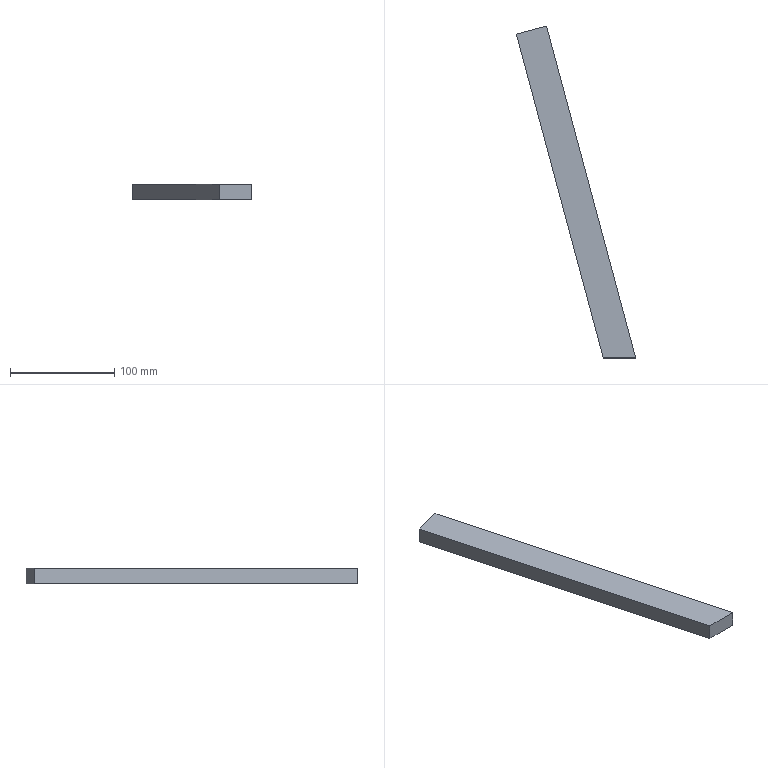Part | NX | features solid 2 | 1 solid | 6 faces | box 114.337 x 318.565 x 15 mm | volume 146602 mm3 | plane 6
STEP:
#1=CARTESIAN_POINT('',(-430.083,270.,-115.));
#2=VERTEX_POINT('',#1);
#3=CARTESIAN_POINT('',(-513.362,580.8,-115.));
#4=VERTEX_POINT('',#3);
#5=CARTESIAN_POINT('',(-443.481,320.,-115.));
#6=DIRECTION('',(-0.2588,0.9659,0.));
#7=VECTOR('',#6,1000.);
#8=LINE('',#5,#7);
#9=EDGE_CURVE('',#2,#4,#8,.T.);
#10=ORIENTED_EDGE('',*,*,#9,.F.);
#11=CARTESIAN_POINT('',(-430.083,270.,-100.));
#12=VERTEX_POINT('',#11);
#13=CARTESIAN_POINT('',(-430.083,270.,-100.));
#14=DIRECTION('',(0.,0.,1.));
#15=VECTOR('',#14,1000.);
#16=LINE('',#13,#15);
#17=EDGE_CURVE('',#2,#12,#16,.T.);
#18=ORIENTED_EDGE('',*,*,#17,.T.);
#19=CARTESIAN_POINT('',(-513.362,580.8,-100.));
#20=VERTEX_POINT('',#19);
#21=CARTESIAN_POINT('',(-443.481,320.,-100.));
#22=DIRECTION('',(-0.2588,0.9659,0.));
#23=VECTOR('',#22,1000.);
#24=LINE('',#21,#23);
#25=EDGE_CURVE('',#12,#20,#24,.T.);
#26=ORIENTED_EDGE('',*,*,#25,.T.);
#27=CARTESIAN_POINT('',(-513.362,580.8,-100.));
#28=DIRECTION('',(0.,0.,-1.));
#29=VECTOR('',#28,1000.);
#30=LINE('',#27,#29);
#31=EDGE_CURVE('',#4,#20,#30,.F.);
#32=ORIENTED_EDGE('',*,*,#31,.F.);
#33=EDGE_LOOP('',(#10,#18,#26,#32));
#34=FACE_BOUND('',#33,.T.);
#35=CARTESIAN_POINT('',(-443.481,320.,-115.));
#36=DIRECTION('',(-0.9659,-0.2588,0.));
#37=DIRECTION('',(0.,0.,1.));
#38=AXIS2_PLACEMENT_3D('',#35,#36,#37);
#39=PLANE('',#38);
#40=ADVANCED_FACE('',(#34),#39,.T.);
#41=ORIENTED_EDGE('',*,*,#25,.F.);
#42=CARTESIAN_POINT('',(-399.025,270.,-100.));
#43=VERTEX_POINT('',#42);
#44=CARTESIAN_POINT('',(-442.5,270.,-100.));
#45=DIRECTION('',(1.,0.,0.));
#46=VECTOR('',#45,1000.);
#47=LINE('',#44,#46);
#48=EDGE_CURVE('',#12,#43,#47,.T.);
#49=ORIENTED_EDGE('',*,*,#48,.T.);
#50=CARTESIAN_POINT('',(-484.384,588.565,-100.));
#51=VERTEX_POINT('',#50);
#52=CARTESIAN_POINT('',(-414.503,327.765,-100.));
#53=DIRECTION('',(-0.2588,0.9659,0.));
#54=VECTOR('',#53,1000.);
#55=LINE('',#52,#54);
#56=EDGE_CURVE('',#43,#51,#55,.T.);
#57=ORIENTED_EDGE('',*,*,#56,.T.);
#58=CARTESIAN_POINT('',(-513.362,580.8,-100.));
#59=DIRECTION('',(-0.9659,-0.2588,0.));
#60=VECTOR('',#59,1000.);
#61=LINE('',#58,#60);
#62=EDGE_CURVE('',#20,#51,#61,.F.);
#63=ORIENTED_EDGE('',*,*,#62,.F.);
#64=EDGE_LOOP('',(#41,#49,#57,#63));
#65=FACE_BOUND('',#64,.T.);
#66=CARTESIAN_POINT('',(-443.481,320.,-100.));
#67=DIRECTION('',(0.,0.,1.));
#68=DIRECTION('',(0.9659,0.2588,0.));
#69=AXIS2_PLACEMENT_3D('',#66,#67,#68);
#70=PLANE('',#69);
#71=ADVANCED_FACE('',(#65),#70,.T.);
#72=ORIENTED_EDGE('',*,*,#56,.F.);
#73=CARTESIAN_POINT('',(-399.025,270.,-115.));
#74=VERTEX_POINT('',#73);
#75=CARTESIAN_POINT('',(-399.025,270.,-115.));
#76=DIRECTION('',(0.,0.,-1.));
#77=VECTOR('',#76,1000.);
#78=LINE('',#75,#77);
#79=EDGE_CURVE('',#74,#43,#78,.F.);
#80=ORIENTED_EDGE('',*,*,#79,.F.);
#81=CARTESIAN_POINT('',(-484.384,588.565,-115.));
#82=VERTEX_POINT('',#81);
#83=CARTESIAN_POINT('',(-414.503,327.765,-115.));
#84=DIRECTION('',(-0.2588,0.9659,0.));
#85=VECTOR('',#84,1000.);
#86=LINE('',#83,#85);
#87=EDGE_CURVE('',#74,#82,#86,.T.);
#88=ORIENTED_EDGE('',*,*,#87,.T.);
#89=CARTESIAN_POINT('',(-484.384,588.565,-115.));
#90=DIRECTION('',(0.,0.,1.));
#91=VECTOR('',#90,1000.);
#92=LINE('',#89,#91);
#93=EDGE_CURVE('',#82,#51,#92,.T.);
#94=ORIENTED_EDGE('',*,*,#93,.T.);
#95=EDGE_LOOP('',(#72,#80,#88,#94));
#96=FACE_BOUND('',#95,.T.);
#97=CARTESIAN_POINT('',(-414.503,327.765,-115.));
#98=DIRECTION('',(-0.9659,-0.2588,0.));
#99=DIRECTION('',(0.,0.,1.));
#100=AXIS2_PLACEMENT_3D('',#97,#98,#99);
#101=PLANE('',#100);
#102=ADVANCED_FACE('',(#96),#101,.F.);
#103=CARTESIAN_POINT('',(-443.481,270.,-115.));
#104=DIRECTION('',(-1.,0.,0.));
#105=VECTOR('',#104,1000.);
#106=LINE('',#103,#105);
#107=EDGE_CURVE('',#2,#74,#106,.F.);
#108=ORIENTED_EDGE('',*,*,#107,.F.);
#109=ORIENTED_EDGE('',*,*,#9,.T.);
#110=CARTESIAN_POINT('',(-513.362,580.8,-115.));
#111=DIRECTION('',(0.9659,0.2588,0.));
#112=VECTOR('',#111,1000.);
#113=LINE('',#110,#112);
#114=EDGE_CURVE('',#4,#82,#113,.T.);
#115=ORIENTED_EDGE('',*,*,#114,.T.);
#116=ORIENTED_EDGE('',*,*,#87,.F.);
#117=EDGE_LOOP('',(#108,#109,#115,#116));
#118=FACE_BOUND('',#117,.T.);
#119=CARTESIAN_POINT('',(-443.481,320.,-115.));
#120=DIRECTION('',(0.,0.,1.));
#121=DIRECTION('',(0.9659,0.2588,0.));
#122=AXIS2_PLACEMENT_3D('',#119,#120,#121);
#123=PLANE('',#122);
#124=ADVANCED_FACE('',(#118),#123,.F.);
#125=ORIENTED_EDGE('',*,*,#93,.F.);
#126=ORIENTED_EDGE('',*,*,#114,.F.);
#127=ORIENTED_EDGE('',*,*,#31,.T.);
#128=ORIENTED_EDGE('',*,*,#62,.T.);
#129=EDGE_LOOP('',(#125,#126,#127,#128));
#130=FACE_BOUND('',#129,.T.);
#131=CARTESIAN_POINT('',(-513.362,580.8,-100.));
#132=DIRECTION('',(0.2588,-0.9659,0.));
#133=DIRECTION('',(0.9659,0.2588,0.));
#134=AXIS2_PLACEMENT_3D('',#131,#132,#133);
#135=PLANE('',#134);
#136=ADVANCED_FACE('',(#130),#135,.F.);
#137=ORIENTED_EDGE('',*,*,#79,.T.);
#138=ORIENTED_EDGE('',*,*,#48,.F.);
#139=ORIENTED_EDGE('',*,*,#17,.F.);
#140=ORIENTED_EDGE('',*,*,#107,.T.);
#141=EDGE_LOOP('',(#137,#138,#139,#140));
#142=FACE_BOUND('',#141,.T.);
#143=CARTESIAN_POINT('',(-442.5,270.,-100.));
#144=DIRECTION('',(0.,1.,0.));
#145=DIRECTION('',(0.,0.,1.));
#146=AXIS2_PLACEMENT_3D('',#143,#144,#145);
#147=PLANE('',#146);
#148=ADVANCED_FACE('',(#142),#147,.F.);
#149=CLOSED_SHELL('',(#40,#71,#102,#124,#136,#148));
#150=MANIFOLD_SOLID_BREP('',#149);
#151=(LENGTH_UNIT()NAMED_UNIT(*)SI_UNIT(.MILLI.,.METRE.));
#152=UNCERTAINTY_MEASURE_WITH_UNIT(LENGTH_MEASURE(0.00001),#151,'','');
#153=(NAMED_UNIT(*)PLANE_ANGLE_UNIT()SI_UNIT($,.RADIAN.));
#154=(NAMED_UNIT(*)SI_UNIT($,.STERADIAN.)SOLID_ANGLE_UNIT());
#155=(GEOMETRIC_REPRESENTATION_CONTEXT(3)GLOBAL_UNCERTAINTY_ASSIGNED_CONTEXT((#152))GLOBAL_UNIT_ASSIGNED_CONTEXT((#151,#153,#154))REPRESENTATION_CONTEXT('',''));
#156=ADVANCED_BREP_SHAPE_REPRESENTATION('',(#150),#155);